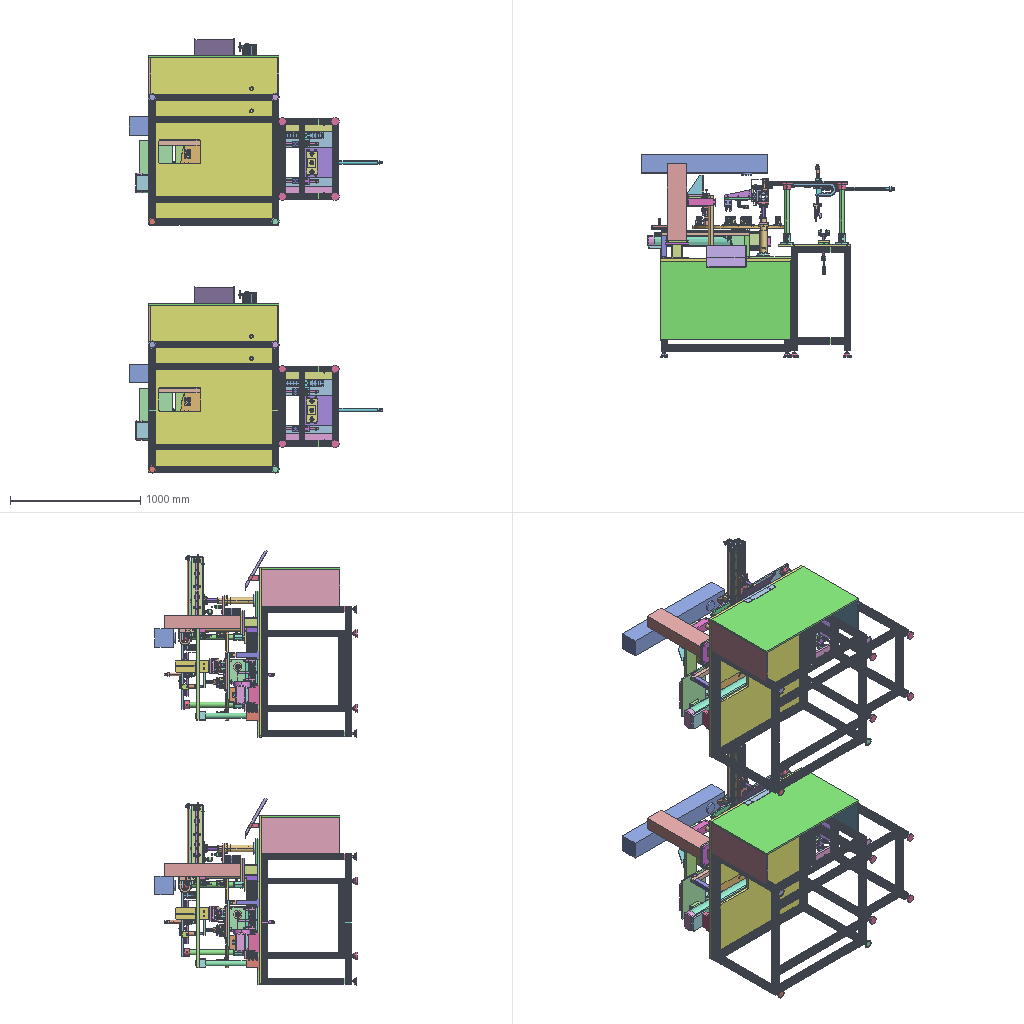Assembly | STEP file | 109 different items | 370 placed | box 1945 x 1552 x 3333 mm
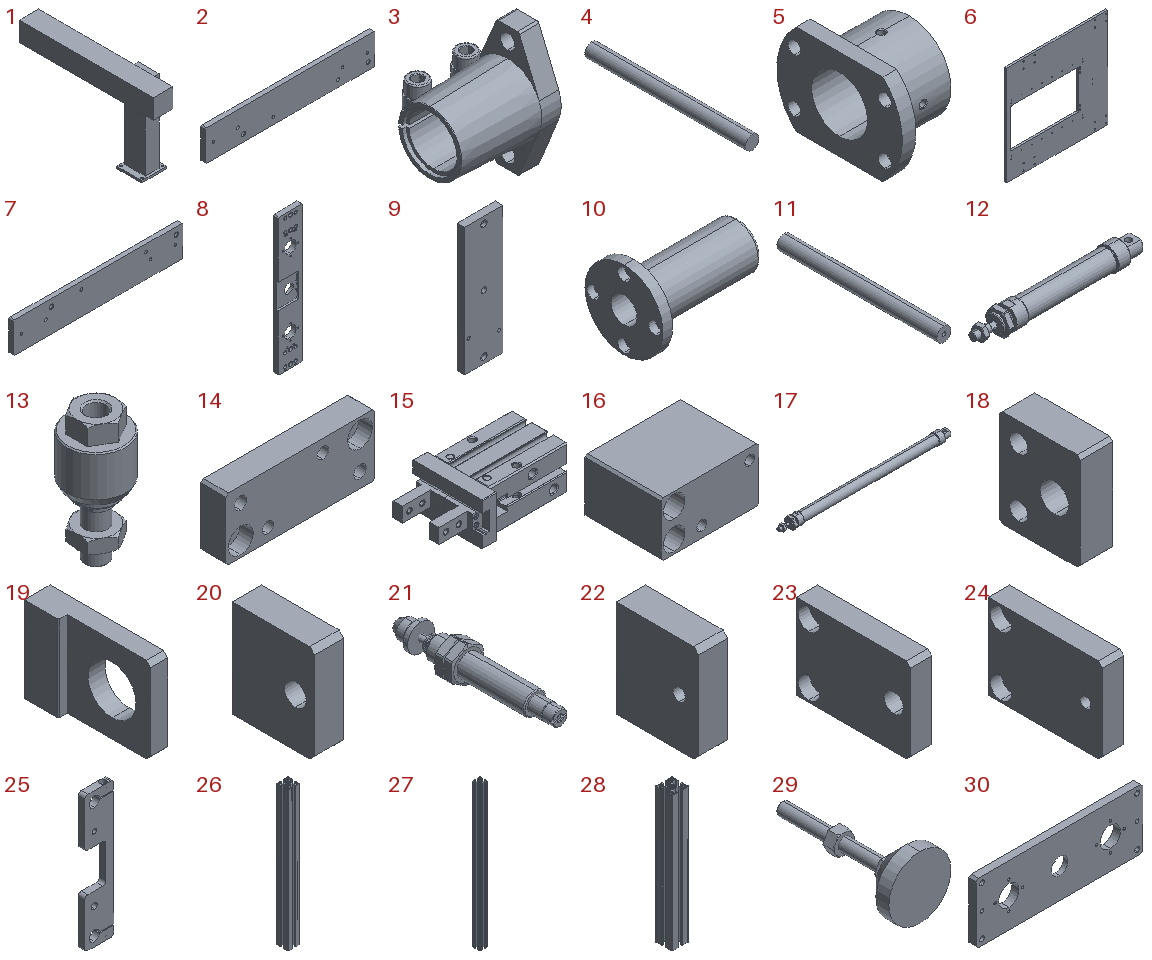Parts list (item | name | quantity | parent item | size | volume):
1 | Ultrasonic welding | x2 | - | 280 x 970 x 675 mm | 28415691 mm3
2 | PN_0058 | x2 | in PN_0042 | 550 x 15 x 100 mm | 808868 mm3
3 | SHFML40 | x8 | in PN_0042 | 80 x 67 x 102 mm | 113573 mm3
4 | PSFJ40-470 | x8 | in PN_0042 | 40 x 470 x 40 mm | 590619 mm3
5 | sthc40 | x8 | in PN_0042 | 50 x 90 x 65 mm | 100252 mm3
6 | PN_0008 | x2 | in PN_0042 | 600 x 12 x 585 mm | 3092667 mm3
7 | PN_0057 | x2 | in PN_0042 | 550 x 15 x 100 mm | 808868 mm3
8 | PN_0025 | x2 | in PN_0042 | 60 x 12 x 335 mm | 203956 mm3
9 | PN_0018 | x2 | in PN_0042 | 60 x 12 x 200 mm | 140928 mm3
10 | LHFRW16 | x4 | in PN_0042 | 70 x 48 x 48 mm | 35245 mm3
11 | PSFJW16-180-M5-N5 | x4 | in PN_0042 | 16 x 180 x 16 mm | 35836 mm3
12 | MA25x75-S (0) | x2 | in PN_0042 | - | -
13 | F-M10125F | x4 | in PN_0042 | 26 x 26 x 58 mm | 16271 mm3
14 | PN_0033 | x2 | in PN_0042 | 60 x 10 x 25 mm | 12893 mm3
15 | HFZ16-CL | x4 | in PN_0042 | 67.3 x 38 x 23.6 mm | 30935 mm3
16 | PN_0049 | x2 | in PN_0042 | 45 x 35 x 25 mm | 32071 mm3
17 | MA25x350-S (0) | x2 | in PN_0042 | - | -
18 | PN_0052 | x2 | in PN_0042 | 10 x 25 x 30 mm | 5805 mm3
19 | PN_0027 | x2 | in PN_0042 | 12 x 55 x 40 mm | 16587 mm3
20 | PN_0024 | x2 | in PN_0042 | 12 x 34 x 40 mm | 15028 mm3
21 | ACJ-1007 | x6 | in PN_0042 | - | -
22 | PN_0037 | x2 | in PN_0042 | 12 x 34 x 40 mm | 15555 mm3
23 | PN_0007 | x2 | in PN_0042 | 10 x 54 x 40 mm | 19857 mm3
24 | PN_0015 | x2 | in PN_0042 | 10 x 54 x 40 mm | 20297 mm3
25 | PN_0034 | x2 | in PN_0042 | 45 x 10 x 210 mm | 67263 mm3
26 | PN_0041 | x10 | in PN_0003 | 45 x 45 x 530 mm | 340057 mm3
27 | PN_0017 | x8 | in PN_0003 | 45 x 45 x 800 mm | 513293 mm3
28 | PN_0029 | x8 | in PN_0003 | 45 x 45 x 360 mm | 230982 mm3
29 | FBR60-12-100 | x8 | in PN_0003 | 60 x 133 x 60 mm | 73980 mm3
30 | PN_0016 | x2 | in PN_0028 | 230 x 10 x 83 mm | 156846 mm3
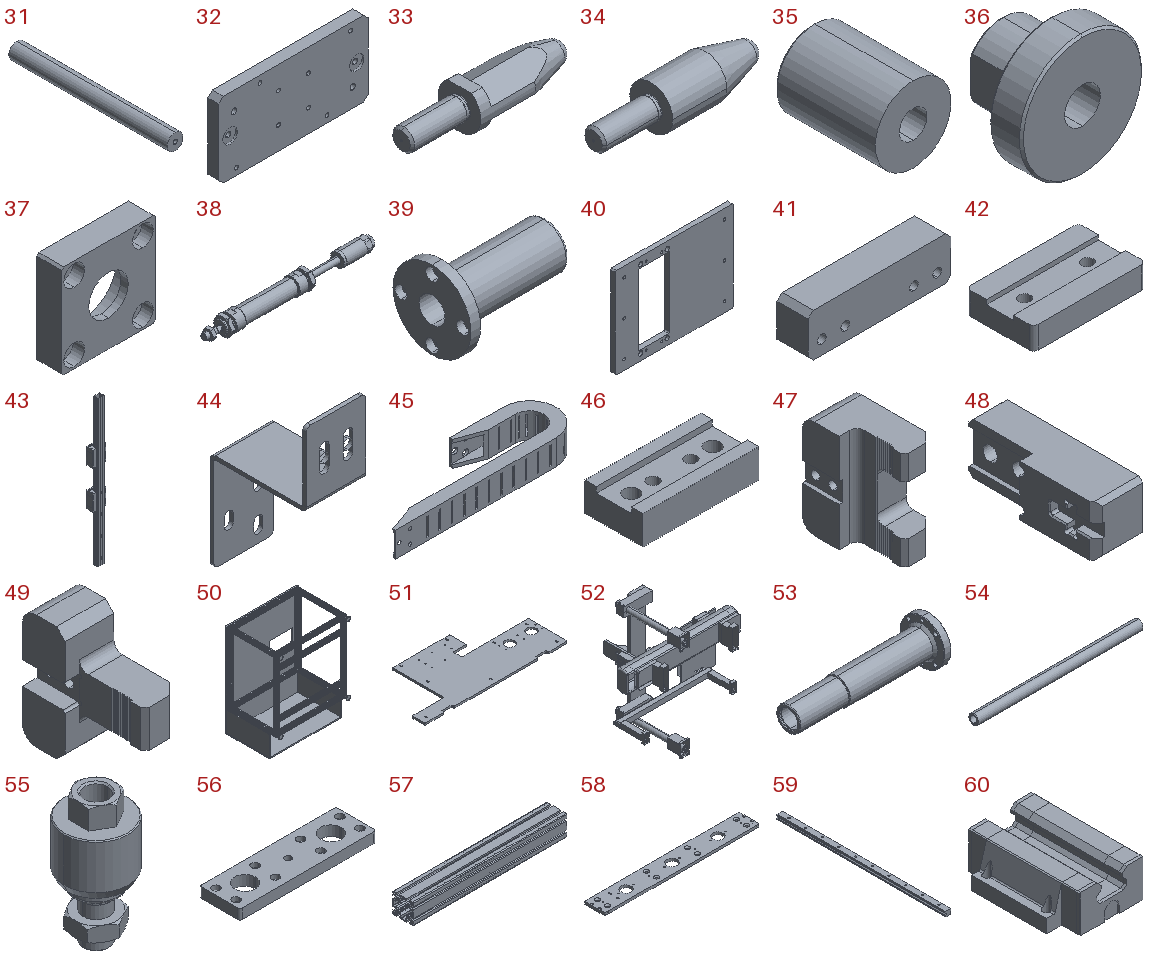31 | PSFJW16-160-M5-N5 | x4 | in PN_0028 | 16 x 160 x 16 mm | 31815 mm3
32 | PN_0056 | x2 | in PN_0028 | 165 x 12 x 83 mm | 159860 mm3
33 | FLNND6_P11_8_B15_0_L10_FLNND6-P11.8-B15.0-L10 | x2 | in PN_0028 | 44.415 x 11.8 x 10.8 mm | 2279 mm3
34 | FLNNA6_P11_9_B15_0_L10---2_FLNNA6-P11.9-B15.0-L10 | x2 | in PN_0028 | 44.601 x 11.9 x 11.9 mm | 2879 mm3
35 | PN_0011 | x8 | in PN_0028 | 15 x 20 x 15 mm | 2655 mm3
36 | PN_0022 | x2 | in PN_0028 | 30 x 20 x 30 mm | 7262 mm3
37 | PN_0055 | x2 | in PN_0028 | 45 x 12 x 45 mm | 14544 mm3
38 | MAJ-25x50-30-S (0300) | x2 | in PN_0028 | - | -
39 | LHFRW16-2 | x4 | in PN_0028 | 70 x 48 x 48 mm | 35245 mm3
40 | PN_0021 | x2 | in PN_0042 | 300 x 12 x 230 mm | 646136 mm3
41 | PN_0043 | x4 | in PN_0042 | 83 x 18 x 25 mm | 35337 mm3
42 | PN_0044 | x2 | in PN_0042 | 50 x 30 x 10 mm | 13429 mm3
43 | EHG20SA | x4 | in PN_0042 | - | -
44 | PN_0005 | x2 | in PN_0042 | - | -
45 | TP18.35(Ruiao) | x2 | in PN_0042 | 349.5 x 99 x 47 mm | 205052 mm3
46 | PN_0031 | x4 | in PN_0042 | 40 x 20 x 10 mm | 6491 mm3
47 | PN_0053 | x2 | in PN_0042 | 19.2 x 35 x 39.94 mm | 17498 mm3
48 | PN_0051 | x4 | in PN_0042 | 11 x 33 x 12 mm | 3442 mm3
49 | PN_0002 | x2 | in PN_0042 | 17 x 38.5 x 40 mm | 12649 mm3
50 | Final inspection modification | x2 | - | 1005 x 750 x 1303 mm | 47486474 mm3
51 | PN_0001 | x2 | - | 1120 x 505 x 15 mm | 5379555 mm3
52 | PN_0054 | x2 | - | - | -
53 | PN_0061_Default<machined> | x4 | in PN_0020 | 292 x 92 x 92 mm | 411633 mm3
54 | PSPJ30_X_PSPJ25-400 | x4 | in PN_0020 | 500 x 30 x 30 mm | 196257 mm3
55 | F_M14150F_F-M14150F-P | x2 | in PN_0020 | 34.5 x 34.5 x 70 mm | 35537 mm3
56 | PN_0006 | x2 | in PN_0020 | 270 x 80 x 20 mm | 358346 mm3
57 | PN_0062_Default<machined> | x2 | in PN_0020 | 606 x 80 x 80 mm | 921943 mm3
58 | PN_0050 | x2 | in PN_0020 | 606 x 80 x 10 mm | 436139 mm3
59 | HGW20CC guide rail-x1 | x2 | in PN_0020 | 20 x 606 x 17.5 mm | 184749 mm3
60 | HGW20CC | x2 | in PN_0020 | 63 x 75 x 25.4 mm | 76452 mm3
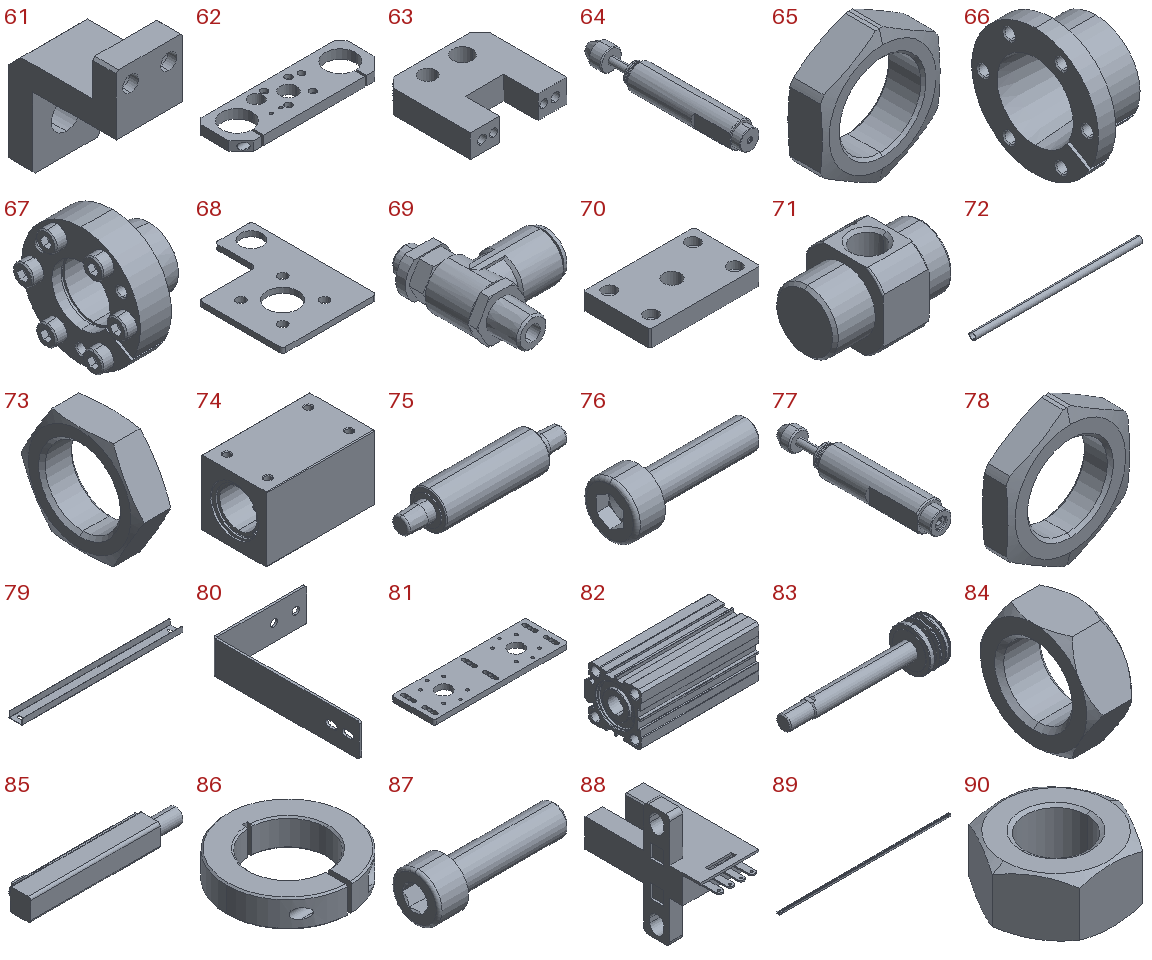61 | PN_0030 | x2 | in PN_0020 | 28 x 45 x 55 mm | 22140 mm3
62 | PN_0048 | x2 | in PN_0020 | 240 x 76 x 15 mm | 181438 mm3
63 | PN_0010 | x4 | in PN_0020 | 50 x 45 x 12 mm | 17113 mm3
64 | ACA_1412_1_Body | x6 | in ACA_1412_1_ACA-1412-1 | 14 x 90 x 14 mm | 10670 mm3
65 | ACA_1412_1_NT | x12 | in ACA_1412_1_ACA-1412-1 | 19 x 6 x 21.289 mm | 1012 mm3
66 | MLR30body | x4 | in MLR30_MLR30 | 28 x 58.56 x 58.56 mm | 23041 mm3
67 | MLR30bonnet | x4 | in MLR30_MLR30 | 41 x 61 x 61 mm | 20958 mm3
68 | PN_0060 | x4 | in PN_0020 | 90 x 120 x 5 mm | 36578 mm3
69 | SPCNL8_1_B_SPCNL8-1-B | x4 | in PN_0020 | 32.883 x 41.9 x 15 mm | 6567 mm3
70 | PN_0035 | x2 | in PN_0020 | 66 x 40 x 10 mm | 24322 mm3
71 | RMS20X50_FCV | x4 | - | 38 x 25 x 25 mm | 12617 mm3
72 | - | x2 | - | 576 x 23 x 23 mm | 58326 mm3
73 | RMS20X50_Nut | x4 | - | 8 x 30.022 x 26 mm | 2480 mm3
74 | RMS20X50_Body | x4 | in PN_0020 | 66 x 40 x 40 mm | 76860 mm3
75 | RMS20X50_Piston | x2 | - | 86 x 20 x 20 mm | 19878 mm3
76 | hexagon socket head cap screws gb_PreviewCfg | x8 | in PN_0020 | 7.6 x 3 x 3 mm | 21.652 mm3
77 | ACA_1210_1_Body | x4 | in ACA_1210_1_ACA-1210-1 | 12 x 67 x 12 mm | 5400 mm3
78 | ACA_1210_1_NT | x8 | in ACA_1210_1_ACA-1210-1 | 17 x 4 x 19.048 mm | 576.274 mm3
79 | PN_0040 | x2 | in PN_0020 | 580 x 47.4 x 21.2 mm | 59564 mm3
80 | PN_0032 | x2 | in PN_0020 | 84 x 134 x 30 mm | 12571 mm3
81 | PN_0036 | x2 | in PN_0020 | - | -
82 | ACQS_40x8080_b | x2 | - | 119.5 x 57 x 53 mm | 166175 mm3
83 | ACQS_40x80_B_80r | x2 | - | 143 x 40 x 40 mm | 43643 mm3
84 | ACQ_40_Nut | x2 | - | 8 x 21.939 x 19 mm | 1486 mm3
85 | CS1_G | x4 | - | 30.5 x 5.5 x 4.4 mm | 552.742 mm3
86 | SCSJ50_18b | x2 | in SCSJ50_18_SCSJ50-18 | 80 x 79.972 x 18 mm | 50835 mm3
87 | - | x2 | in SCSJ50_18_SCSJ50-18 | 38 x 13 x 13 mm | 2398 mm3
88 | EE-SX672-D12d(Omron U-shaped photoelectric) | x4 | in PN_0020 | 13.5 x 28.5 x 26 mm | 1979 mm3
89 | SENAK3-X | x2 | in PN_0020 | 606 x 9 x 6 mm | 19051 mm3
90 | hex nuts 1-fine pitch-grades ab gb_PreviewCfg | x2 | in PN_0020 | 18.475 x 16 x 8.4 mm | 1301 mm3
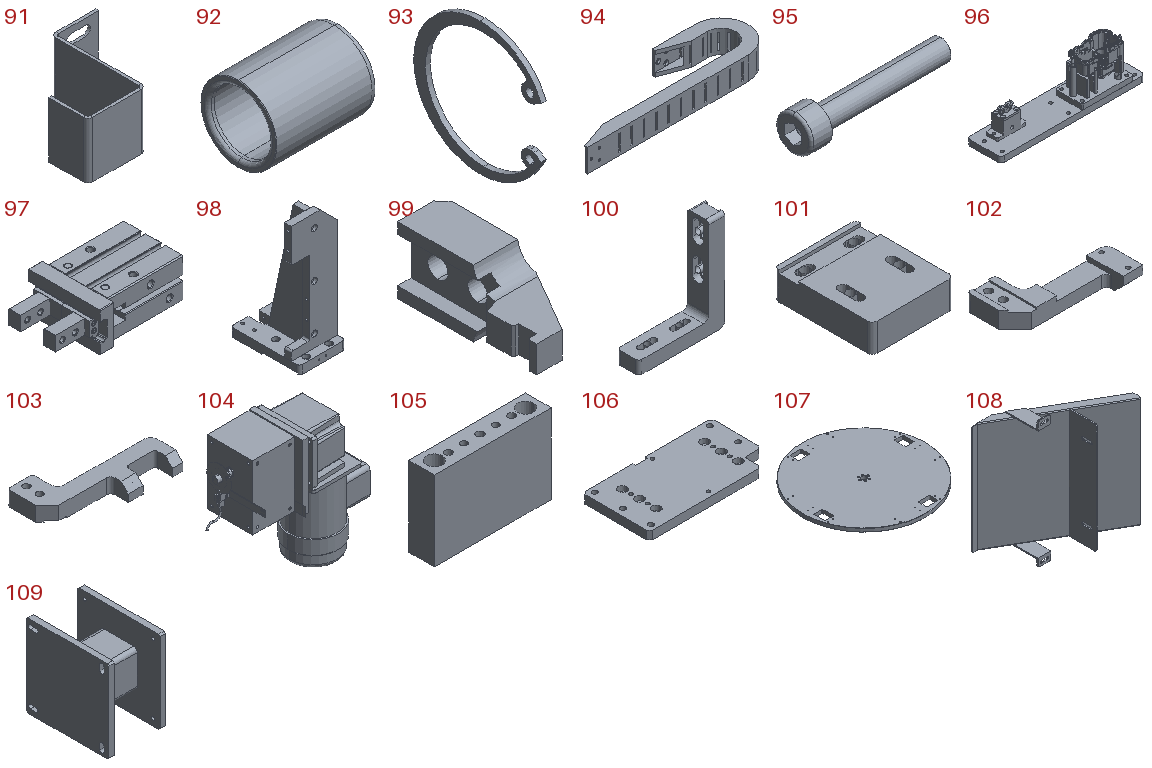91 | PN_0038 | x2 | in PN_0020 | 35.75 x 33 x 20 mm | 1529 mm3
92 | MPBZ30_50_MPBZ30-50 | x8 | in PN_0020 | 50 x 38 x 38 mm | 21031 mm3
93 | RTWN37_RTWN37 | x8 | in PN_0020 | 1.5 x 38.283 x 39.8 mm | 431.748 mm3
94 | TP15.30(Ruiao) | x2 | in PN_0020 | 349.5 x 99 x 43 mm | 233329 mm3
95 | GB_Hex socket head cylinder screw_M5X30_M5X30 | x2 | in PN_0020 | 35 x 8.5 x 8.5 mm | 830.962 mm3
96 | PN_0047 | x10 | in PN_0020, Turntable carrier | - | -
97 | HFZ20_CL_ | x4 | in PN_0020 | 84.7 x 50 x 27.6 mm | 63972 mm3
98 | PN_0013 | x2 | in PN_0020 | 80 x 120 x 219 mm | 332786 mm3
99 | PN_0004 | x4 | in PN_0020 | 13.8 x 35 x 15 mm | 2765 mm3
100 | PN_0023 | x2 | in PN_0020 | - | -
101 | PN_0019 | x2 | in PN_0020 | - | -
102 | PN_0059 | x2 | in PN_0020 | 67.5 x 39 x 10 mm | 9820 mm3
103 | PN_0045 | x2 | in PN_0020 | 80 x 39 x 10 mm | 11727 mm3
104 | PN_0046 | x2 | in PN_0014 | - | -
105 | PN_0026 | x4 | in PN_0014 | 110 x 24 x 75 mm | 174240 mm3
106 | PN_0012 | x2 | in PN_0014 | 230 x 120 x 15 mm | 374023 mm3
107 | PN_0009 | x2 | in Turntable carrier | 700 x 700 x 20 mm | 7409055 mm3
108 | PN_0039 | x2 | - | 305 x 168 x 349 mm | 258678 mm3
109 | PN_0063_Default<machined> | x2 | - | 124 x 180 x 180 mm | 884667 mm3
Placements (level | parent | child | x y z in mm | rotation matrix by rows), first 340 of 402 lines:
1 | subassembly 2 | Ultrasonic welding | -163.522 990.0 690.769 | 0 1 0 0 0 1 1 0 0
1 | subassembly 2 | PN_0042 | 719.818 434.3 178.269 | 1 0 0 0 1 0 0 0 1
2 | PN_0042 | PN_0058 | -40.835 -5.8 -0.0 | 1 0 0 0 1 0 0 0 1
2 | PN_0042 | SHFML40 | 169.165 9.2 -0.0 | 0 0 -1 -1 0 0 0 1 0
2 | PN_0042 | PSFJ40-470 | 169.165 9.2 0.0 | 0.9999 0 -0.01343 0 1 0 0.01343 0 0.9999
2 | PN_0042 | sthc40 | 169.165 479.2 -0.0 | 0 1 0 -1 0 0 0 0 1
2 | PN_0042 | PN_0008 | -85.835 479.2 260.0 | 1 0 0 0 1 0 0 0 1
2 | PN_0042 | PN_0057 | -40.835 -5.8 520.0 | 1 0 0 0 1 0 0 0 1
2 | PN_0042 | PN_0025 | -14.335 451.2 232.5 | 1 0 0 0 1 0 0 0 1
2 | PN_0042 | PN_0018 | -14.335 322.2 232.5 | 1 0 0 0 1 0 0 0 1
2 | PN_0042 | LHFRW16 | -14.335 457.2 322.5 | 0 1 0 -1 0 0 0 0 1
2 | PN_0042 | PSFJW16-180-M5-N5 | -14.335 320.2 322.5 | 0.998 0 -0.06356 0 1 0 0.06356 0 0.998
2 | PN_0042 | MA25x75-S (0) | -14.335 467.2 232.5 | 0 0 1 1 0 0 0 1 0
2 | PN_0042 | F-M10125F | -14.335 357.2 232.5 | 0.7177 0.6964 0 0 0 1 0.6964 -0.7177 0
2 | PN_0042 | PN_0033 | -14.335 300.2 173.0 | 1 0 0 0 1 0 0 0 1
2 | PN_0042 | HFZ16-CL | -16.335 300.2 173.0 | 0 1 0 1 0 0 0 0 -1
2 | PN_0042 | HFZ16-CL | -28.835 275.2 308.7 | 0 0 1 1 0 0 0 1 -0
2 | PN_0042 | PN_0049 | -28.835 275.2 301.5 | 0 0 -1 0 1 0 1 0 0
2 | PN_0042 | MA25x350-S (0) | 145.165 434.2 232.5 | 1 0 0 0 -0.8525 0.5227 0 -0.5227 -0.8525
2 | PN_0042 | F-M10125F | 17.665 434.2 232.5 | 0 0 1 -0.03816 -0.9993 0 0.9993 -0.03816 -0
2 | PN_0042 | PN_0052 | 15.665 438.7 232.5 | 1 0 0 0 1 0 0 0 1
2 | PN_0042 | PN_0027 | 123.165 471.2 232.5 | 1 0 0 0 1 0 0 0 1
2 | PN_0042 | PN_0024 | 48.165 471.2 137.5 | 1 0 0 0 1 0 0 0 1
2 | PN_0042 | ACJ-1007 | 81.165 445.2 137.5 | 0 -1 0 0.5268 0 -0.85 0.85 0 0.5268
2 | PN_0042 | PN_0037 | 48.165 471.2 327.5 | 1 0 0 0 1 0 0 0 1
2 | PN_0042 | PN_0007 | -395.835 464.2 137.5 | 1 0 0 0 1 0 0 0 1
2 | PN_0042 | PN_0015 | -395.835 464.2 327.5 | 1 0 0 0 1 0 0 0 1
2 | PN_0042 | ACJ-1007 | -429.835 445.2 137.5 | 0 1 0 0.7993 0 -0.601 -0.601 0 -0.7993
2 | PN_0042 | PN_0034 | -4.335 500.2 232.5 | 1 0 0 0 1 0 0 0 1
2 | PN_0042 | ACJ-1007 | -14.335 515.7 182.5 | 0.986 0 0.1665 0 -1 0 0.1665 0 -0.986
2 | PN_0042 | PN_0003 | 202.398 -37.946 260.0 | 1 0 0 0 1 0 0 0 1
3 | PN_0003 | PN_0041 | -1444.398 -532.32 -265.0 | 1 0 0 0 1 0 0 0 1
3 | PN_0003 | PN_0017 | 551.233 32.146 -1166.165 | 0 -1 0 0 0 -1 1 0 0
3 | PN_0003 | PN_0029 | -13.233 -532.32 -1166.165 | 0 0 -1 0 1 0 1 0 0
3 | PN_0003 | PN_0017 | 551.233 32.146 -1741.165 | 0 -1 0 0 0 -1 1 0 0
3 | PN_0003 | PN_0017 | 146.233 32.146 -1166.165 | 0 -1 0 0 0 -1 1 0 0
3 | PN_0003 | PN_0041 | -1849.398 -577.32 -265.0 | 1 0 0 0 1 0 0 0 1
3 | PN_0003 | PN_0029 | -13.233 -532.32 -1741.165 | 0 0 -1 0 1 0 1 0 0
3 | PN_0003 | PN_0017 | 146.233 32.146 -1741.165 | 0 -1 0 0 0 -1 1 0 0
3 | PN_0003 | PN_0041 | -1444.398 -1237.32 -265.0 | 1 0 0 0 1 0 0 0 1
3 | PN_0003 | PN_0041 | -1849.398 -1237.32 -265.0 | 1 0 0 0 1 0 0 0 1
3 | PN_0003 | PN_0029 | -13.233 -1237.32 -1166.165 | 0 0 -1 0 1 0 1 0 0
3 | PN_0003 | PN_0029 | -13.233 -1237.32 -1741.165 | 0 0 -1 0 1 0 1 0 0
3 | PN_0003 | FBR60-12-100 | 9.267 -817.854 287.5 | 1 0 0 0 1 0 0 0 1
3 | PN_0003 | FBR60-12-100 | 9.267 -817.854 -287.5 | 1 0 0 0 1 0 0 0 1
3 | PN_0003 | FBR60-12-100 | -395.733 -817.854 -287.5 | 1 0 0 0 1 0 0 0 1
3 | PN_0003 | FBR60-12-100 | -395.733 -817.854 287.5 | 1 0 0 0 1 0 0 0 1
3 | PN_0003 | PN_0041 | -1699.398 -532.32 -265.0 | 1 0 0 0 1 0 0 0 1
2 | PN_0042 | PN_0028 | 37.301 24.755 239.519 | 0 0 -1 0 1 0 1 0 0
3 | PN_0028 | PN_0016 | -9.019 -0.5551 5.136 | 1 0 0 0 1 0 0 0 1
3 | PN_0028 | PSFJW16-160-M5-N5 | 60.981 -102.555 5.136 | 1 0 0 0 1 0 0 0 1
3 | PN_0028 | PSFJW16-160-M5-N5 | -79.019 -102.555 5.136 | 1 0 0 0 1 0 0 0 1
3 | PN_0028 | PN_0056 | -9.019 55.445 5.136 | 1 0 0 0 1 0 0 0 1
3 | PN_0028 | FLNND6_P11_8_B15_0_L10_FLNND6-P11.8-B15.0-L10 | 56.481 67.445 -15.864 | 0 -1 0 1 0 0 0 0 1
3 | PN_0028 | FLNNA6_P11_9_B15_0_L10---2_FLNNA6-P11.9-B15.0-L10 | -74.519 67.445 26.137 | 0 -1 0 1 0 0 0 0 1
3 | PN_0028 | PN_0011 | 27.981 67.445 -28.863 | 1 0 0 0 1 0 0 0 1
3 | PN_0028 | PN_0011 | -46.019 67.445 39.136 | 1 0 0 0 1 0 0 0 1
3 | PN_0028 | PN_0011 | -72.019 67.445 -28.863 | 1 0 0 0 1 0 0 0 1
3 | PN_0028 | PN_0011 | 53.981 67.445 39.136 | 1 0 0 0 1 0 0 0 1
3 | PN_0028 | PN_0022 | -9.019 55.445 5.136 | 0.7332 0 0.68 0 -1 0 0.68 0 -0.7332
3 | PN_0028 | PN_0055 | -9.019 43.445 5.136 | 1 0 0 0 1 0 0 0 1
3 | PN_0028 | MAJ-25x50-30-S (0300) | -9.019 -16.555 5.136 | 0 0 -1 -1 0 0 0 1 0
3 | PN_0028 | LHFRW16-2 | 60.981 15.445 5.136 | 0 1 0 -1 0 0 0 0 1
3 | PN_0028 | LHFRW16-2 | -79.019 15.445 5.136 | 0 1 0 -1 0 0 0 0 1
2 | PN_0042 | PN_0021 | 84.165 -5.8 230.5 | 1 0 0 0 1 0 0 0 1
2 | PN_0042 | PN_0043 | 32.165 6.2 333.0 | 1 0 0 0 1 0 0 0 1
2 | PN_0042 | PN_0043 | 32.165 6.2 128.0 | -1 0 0 0 1 0 0 0 -1
2 | PN_0042 | PN_0044 | 123.165 479.2 232.5 | 0 1 0 0 0 -1 -1 0 -0
2 | PN_0042 | EHG20SA | -434.835 472.098 376.317 | 0 0 -1 0 -1 0 -1 0 -0
2 | PN_0042 | EHG20SA | -434.835 472.098 91.317 | 0 0 -1 0 -1 0 -1 0 -0
2 | PN_0042 | PN_0005 | -4.335 406.7 397.5 | 1 0 0 0 -1 0 0 0 -1
2 | PN_0042 | TP18.35(Ruiao) | -224.335 467.7 440.5 | 1 0 0 0 -1 0 0 0 -1
2 | PN_0042 | PN_0031 | 48.165 479.2 327.5 | 0 -1 0 0 0 -1 1 0 -0
2 | PN_0042 | PN_0031 | 48.165 479.2 137.5 | 0 -1 0 0 0 -1 1 0 -0
2 | PN_0042 | SHFML40 | -250.835 9.2 0.0 | 0 0 -1 -1 0 0 0 1 0
2 | PN_0042 | SHFML40 | 169.165 9.2 520.0 | 0 0 -1 -1 0 0 0 1 0
2 | PN_0042 | SHFML40 | -250.835 9.2 520.0 | 0 0 -1 -1 0 0 0 1 0
2 | PN_0042 | sthc40 | -250.835 479.2 -0.0 | 0 1 0 -1 0 0 0 0 1
2 | PN_0042 | sthc40 | 169.165 479.2 520.0 | 0 1 0 -1 0 0 0 0 1
2 | PN_0042 | sthc40 | -250.835 479.2 520.0 | 0 1 0 -1 0 0 0 0 1
2 | PN_0042 | PSFJ40-470 | -250.835 9.2 0.0 | 0.9999 0 -0.01343 0 1 0 0.01343 0 0.9999
2 | PN_0042 | PSFJ40-470 | 169.165 9.2 520.0 | 0.9999 0 -0.01343 0 1 0 0.01343 0 0.9999
2 | PN_0042 | PSFJ40-470 | -250.835 9.2 520.0 | 0.9999 0 -0.01343 0 1 0 0.01343 0 0.9999
2 | PN_0042 | PN_0053 | -5.375 232.9 173.03 | 1 0 0 0 1 0 0 0 1
2 | PN_0042 | PN_0051 | -28.835 222.9 326.16 | 0 0 -1 0 1 0 1 0 0
2 | PN_0042 | PN_0002 | -21.595 232.9 173.0 | -1 0 0 0 1 0 0 0 -1
2 | PN_0042 | PN_0051 | -28.835 222.9 291.24 | 0 0 1 0 1 0 -1 0 -0
2 | PN_0042 | PSFJW16-180-M5-N5 | -14.335 320.2 142.5 | 0.998 0 -0.06356 0 1 0 0.06356 0 0.998
2 | PN_0042 | LHFRW16 | -14.335 457.2 142.5 | 0 1 0 -1 0 0 0 0 1
1 | subassembly 2 | Final inspection modification | -1.017 -32.5 911.769 | -1 0 0 0 1 0 0 0 -1
1 | subassembly 2 | PN_0001 | -1.017 345.0 489.269 | 0 -1 0 0 0 -1 1 0 0
1 | subassembly 2 | PN_0054 | -3.106 32.87 911.769 | -1 0 0 0 1 0 0 0 -1
1 | subassembly 2 | PN_0020 | 288.983 477.954 977.897 | 0 0 1 -1 0 0 0 -1 0
2 | PN_0020 | PN_0061_Default<machined> | -171.046 1.128 -0.0 | 1 0 0 0 1 0 0 0 1
2 | PN_0020 | PN_0061_Default<machined> | -171.046 171.128 0.0 | 1 0 0 0 -1 0 0 0 -1
2 | PN_0020 | PSPJ30_X_PSPJ25-400 | -290.379 171.128 -0.0 | 1 0 0 0 0.9961 0.08866 0 -0.08866 0.9961
2 | PN_0020 | PSPJ30_X_PSPJ25-400 | -290.379 1.128 -0.0 | 1 0 0 0 0.9538 0.3006 0 -0.3006 0.9538
2 | PN_0020 | F_M14150F_F-M14150F-P | -277.629 86.128 0.0 | 0 0 1 -0.9375 -0.3479 0 0.3479 -0.9375 0
2 | PN_0020 | PN_0006 | -290.379 86.128 0.0 | 0 0 1 -1 0 0 0 -1 -0
2 | PN_0020 | PN_0062_Default<machined> | -330.379 -26.872 -0.0 | 0 0 1 -1 0 0 0 -1 0
2 | PN_0020 | PN_0050 | -330.379 -26.872 -40.0 | 0 -1 0 -1 0 0 0 0 -1
2 | PN_0020 | HGW20CC guide rail-x1 | -330.379 -64.372 -80.0 | 1 0 0 0 1 0 0 0 1
2 | PN_0020 | HGW20CC | -330.379 204.605 -80.0 | 1 0 0 0 1 0 0 0 1
2 | PN_0020 | PN_0030 | -153.546 48.128 -0.0 | 0 -1 0 1 0 0 0 0 1
2 | PN_0020 | PN_0048 | -116.046 86.128 4.0 | 0 0 -1 1 0 0 0 -1 0
2 | PN_0020 | PN_0010 | -330.379 264.128 -72.5 | 1 0 0 0 0 1 0 -1 0
2 | PN_0020 | PN_0010 | -330.379 -329.872 -72.5 | 1 0 0 0 0 1 0 -1 0
2 | PN_0020 | ACA_1412_1_ACA-1412-1 | -129.546 48.128 -15.0 | 0 -1 0 0.6019 0 0.7986 -0.7986 0 0.6019
3 | ACA_1412_1_ACA-1412-1 | ACA_1412_1_Body | -0.0 -0.0 -0.0 | 1 0 0 0 1 0 0 0 1
3 | ACA_1412_1_ACA-1412-1 | ACA_1412_1_NT | -0.0 46.5 -0.0 | 1 0 0 0 1 0 0 0 1
3 | ACA_1412_1_ACA-1412-1 | ACA_1412_1_NT | -0.0 52.5 -0.0 | 1 0 0 0 1 0 0 0 1
2 | PN_0020 | MLR30_MLR30 | -254.379 1.128 0.0 | -1 0 0 0 -0.8293 -0.5589 0 -0.5589 0.8293
3 | MLR30_MLR30 | MLR30body | -0.0 -0.0 -0.0 | 1 0 0 0 1 0 0 0 1
3 | MLR30_MLR30 | MLR30bonnet | -0.0 -0.0 -0.0 | 1 0 0 0 1 0 0 0 1
2 | PN_0020 | MLR30_MLR30 | -254.379 171.128 -0.0 | -1 0 0 0 -0.5264 0.8502 0 0.8502 0.5264
3 | MLR30_MLR30 | MLR30body | -0.0 -0.0 -0.0 | 1 0 0 0 1 0 0 0 1
3 | MLR30_MLR30 | MLR30bonnet | -0.0 -0.0 -0.0 | 1 0 0 0 1 0 0 0 1
2 | PN_0020 | PN_0060 | -350.379 276.128 0.0 | 0 -1 0 0 0 1 -1 0 0
2 | PN_0020 | PN_0060 | -350.379 -334.872 0.0 | 0 -1 0 0 0 1 -1 0 0
2 | PN_0020 | SPCNL8_1_B_SPCNL8-1-B | -395.379 268.628 -63.0 | -1 0 0 0 0 -1 0 -1 -0
2 | PN_0020 | SPCNL8_1_B_SPCNL8-1-B | -395.379 -322.372 -63.0 | -1 0 0 0 0 -1 0 -1 -0
2 | PN_0020 | PN_0035 | -395.379 204.605 -55.0 | 0 -1 0 -1 0 0 0 0 -1
2 | PN_0020 | subassembly 3 | -395.379 261.128 -35.0 | 0 -1 0 -1 0 0 0 0 -1
3 | subassembly 3 | RMS20X50_FCV | -0.0 -0.0 -0.0 | 1 0 0 0 1 0 0 0 1
3 | subassembly 3 | subassembly 4 | -0.0 -0.0 -0.0 | 1 0 0 0 1 0 0 0 1
3 | subassembly 3 | RMS20X50_FCV | 576.0 0.0 -0.0 | -1 0 0 0 -1 0 0 0 1
3 | subassembly 3 | RMS20X50_Nut | 599.0 0.0 -0.0 | -1 0 0 0 -1 0 0 0 1
3 | subassembly 3 | RMS20X50_Body | 5.0 0.0 -0.0 | 1 0 0 0 1 0 0 0 1
3 | subassembly 3 | RMS20X50_Piston | 10.0 0.0 -0.0 | 1 0 0 0 1 0 0 0 1
3 | subassembly 3 | RMS20X50_Nut | -23.0 0.0 -0.0 | 1 0 0 0 1 0 0 0 1
2 | PN_0020 | RMS20X50_Body | -395.379 237.605 -35.0 | 0 -1 0 -1 0 0 0 0 -1
2 | PN_0020 | hexagon socket head cap screws gb_PreviewCfg | -395.379 204.605 -92.0 | 0 -0.3327 0.943 0 -0.943 -0.3327 1 0 -0
2 | PN_0020 | ACA_1210_1_ACA-1210-1 | -322.379 299.628 -87.0 | 0.9765 0 0.2154 0 -1 0 0.2154 0 -0.9765
3 | ACA_1210_1_ACA-1210-1 | ACA_1210_1_Body | -0.0 -0.0 -0.0 | 1 0 0 0 1 0 0 0 1
3 | ACA_1210_1_ACA-1210-1 | ACA_1210_1_NT | 0.0 32.5 -0.0 | 1 0 0 0 1 0 0 0 1
3 | ACA_1210_1_ACA-1210-1 | ACA_1210_1_NT | 0.0 36.5 -0.0 | 1 0 0 0 1 0 0 0 1
2 | PN_0020 | ACA_1210_1_ACA-1210-1 | -322.379 -353.372 -87.0 | 0.4428 0 0.8966 0 1 0 -0.8966 0 0.4428
3 | ACA_1210_1_ACA-1210-1 | ACA_1210_1_Body | -0.0 -0.0 -0.0 | 1 0 0 0 1 0 0 0 1
3 | ACA_1210_1_ACA-1210-1 | ACA_1210_1_NT | 0.0 32.5 -0.0 | 1 0 0 0 1 0 0 0 1
3 | ACA_1210_1_ACA-1210-1 | ACA_1210_1_NT | 0.0 36.5 -0.0 | 1 0 0 0 1 0 0 0 1
2 | PN_0020 | hexagon socket head cap screws gb_PreviewCfg | -340.379 232.628 -87.0 | 0 -0.3713 0.9285 1 0 0 0 0.9285 0.3713
2 | PN_0020 | hexagon socket head cap screws gb_PreviewCfg | -340.379 -286.372 -87.0 | 0 -0.6192 0.7853 -1 0 0 0 -0.7853 -0.6192
2 | PN_0020 | PN_0040 | -371.579 -13.872 16.3 | 0 0 -1 -1 0 0 0 1 -0
2 | PN_0020 | PN_0032 | -420.786 229.605 -94.0 | 1 0 0 0 0 1 0 -1 0
2 | PN_0020 | PN_0036 | 120.954 86.128 0.0 | 0 0 1 1 0 0 0 1 0
2 | PN_0020 | hexagon socket head cap screws gb_PreviewCfg | -118.646 122.128 -15.0 | 1 0 0 0 1 0 0 0 1
2 | PN_0020 | ACA_1412_1_ACA-1412-1 | -129.546 48.128 -15.0 | 0 -1 0 1 0 0 0 0 1
3 | ACA_1412_1_ACA-1412-1 | ACA_1412_1_Body | -0.0 -0.0 -0.0 | 1 0 0 0 1 0 0 0 1
3 | ACA_1412_1_ACA-1412-1 | ACA_1412_1_NT | -0.0 46.5 -0.0 | 1 0 0 0 1 0 0 0 1
3 | ACA_1412_1_ACA-1412-1 | ACA_1412_1_NT | -0.0 52.5 -0.0 | 1 0 0 0 1 0 0 0 1
2 | PN_0020 | subassembly 5 | -116.046 86.128 0.0 | 1 0 0 0 1 0 0 0 1
3 | subassembly 5 | ACQS_40x8080_b | -0.0 -0.0 -0.0 | 1 0 0 0 0 -1 0 1 0
3 | subassembly 5 | ACQS_40x80_B_80r | -0.0 -0.0 -0.0 | 1 0 0 0 1 0 0 0 1
3 | subassembly 5 | ACQ_40_Nut | -14.25 -0.0 -0.0 | -1 0 0 0 -1 0 0 0 1
3 | subassembly 5 | CS1_G | 1.0 9.931 21.298 | 1 0 0 0 0.4226 -0.9063 0 0.9063 0.4226
3 | subassembly 5 | CS1_G | 118.5 -9.931 21.298 | -1 0 0 0 -0.4226 0.9063 0 0.9063 0.4226
2 | PN_0020 | SCSJ50_18_SCSJ50-18 | -107.046 1.128 -0.0 | 0 0 1 0 -1 0 1 0 0
3 | SCSJ50_18_SCSJ50-18 | SCSJ50_18b | -0.0 -0.0 -0.0 | 1 0 0 0 1 0 0 0 1
3 | SCSJ50_18_SCSJ50-18 | subassembly 6 | 15.0 -32.0 -0.0 | -1 0 0 0 -1 0 0 0 1
2 | PN_0020 | EE-SX672-D12d(Omron U-shaped photoelectric) | -280.129 118.128 -56.75 | 0 1 0 0 0 -1 -1 0 0
2 | PN_0020 | SENAK3-X | -285.879 176.128 -44.0 | 0 -1 0 -1 0 0 0 0 -1
2 | PN_0020 | EE-SX672-D12d(Omron U-shaped photoelectric) | -280.129 -281.622 -56.75 | 0 1 0 0 0 -1 -1 0 0
2 | PN_0020 | ACA_1412_1_ACA-1412-1 | -129.546 48.128 -15.0 | 0 -1 0 0.8791 0 -0.4767 0.4767 0 0.8791
3 | ACA_1412_1_ACA-1412-1 | ACA_1412_1_Body | -0.0 -0.0 -0.0 | 1 0 0 0 1 0 0 0 1
3 | ACA_1412_1_ACA-1412-1 | ACA_1412_1_NT | -0.0 46.5 -0.0 | 1 0 0 0 1 0 0 0 1
3 | ACA_1412_1_ACA-1412-1 | ACA_1412_1_NT | -0.0 52.5 -0.0 | 1 0 0 0 1 0 0 0 1
2 | PN_0020 | hex nuts 1-fine pitch-grades ab gb_PreviewCfg | -340.379 -317.872 -87.0 | 0.5037 -0.8639 0 0 0 -1 0.8639 0.5037 -0
2 | PN_0020 | PN_0038 | -262.786 204.605 -56.25 | 0 -1 0 0 0 1 -1 0 -0
2 | PN_0020 | MPBZ30_50_MPBZ30-50 | -166.046 1.128 -0.0 | 1 0 0 0 0.7589 0.6512 0 -0.6512 0.7589
2 | PN_0020 | MPBZ30_50_MPBZ30-50 | -166.046 171.128 0.0 | 1 0 0 0 0.2659 0.964 0 -0.964 0.2659
2 | PN_0020 | MPBZ30_50_MPBZ30-50 | 63.954 1.128 0.0 | 1 0 0 0 0.6815 -0.7318 0 0.7318 0.6815
2 | PN_0020 | MPBZ30_50_MPBZ30-50 | 63.954 171.128 0.0 | 1 0 0 0 0.6815 -0.7318 0 0.7318 0.6815
2 | PN_0020 | RTWN37_RTWN37 | -166.896 1.128 -0.0 | 1 0 0 0 0.6761 -0.7368 0 0.7368 0.6761
2 | PN_0020 | RTWN37_RTWN37 | -166.896 171.128 0.0 | 1 0 0 0 0.5147 -0.8574 0 0.8574 0.5147
2 | PN_0020 | RTWN37_RTWN37 | 114.804 1.128 -0.0 | 1 0 0 0 -0.9964 -0.08438 0 0.08438 -0.9964
2 | PN_0020 | RTWN37_RTWN37 | 114.804 171.128 0.0 | 1 0 0 0 -0.9964 -0.08438 0 0.08438 -0.9964
2 | PN_0020 | TP15.30(Ruiao) | -383.079 -5.395 17.3 | 0 -1 0 1 0 0 0 0 1
2 | PN_0020 | GB_Hex socket head cylinder screw_M5X30_M5X30 | -337.554 193.128 -84.5 | 0 -0.2637 -0.9646 1 0 0 0 -0.9646 0.2637
2 | PN_0020 | PN_0047 | -0.2834 815.301 3543.794 | 0 0 -1 0 1 0 1 0 -0
2 | PN_0020 | HFZ20_CL_ | -316.836 273.405 -271.0 | -1 0 0 0 0 -1 0 -1 0
2 | PN_0020 | PN_0013 | -355.786 204.605 -77.0 | 0 -1 0 -1 0 0 0 0 -1
2 | PN_0020 | PN_0004 | -252.136 265.905 -268.41 | 0 -1 0 0 0 1 -1 0 -0
2 | PN_0020 | PN_0004 | -252.136 280.905 -273.59 | 0 -1 0 0 0 -1 1 0 0
2 | PN_0020 | HFZ20_CL_ | -344.786 257.605 -189.2 | -1 0 0 0 1 0 0 0 -1
2 | PN_0020 | PN_0023 | -315.786 250.605 -215.0 | 0 1 0 -1 0 0 0 0 1
2 | PN_0020 | PN_0019 | -294.836 259.605 -271.0 | 0 -1 0 0 0 -1 1 0 0
2 | PN_0020 | PN_0059 | -264.586 282.765 -163.5 | 0 -1 0 0 0 -1 1 0 0
2 | PN_0020 | PN_0045 | -259.586 242.445 -157.25 | 0 -1 0 0 0 -1 1 0 0
1 | subassembly 2 | PN_0014 | 195.047 506.863 362.055 | 1 0 0 0 1 0 0 0 1
2 | PN_0014 | PN_0046 | -99.074 48.137 46.714 | 1 0 0 0 1 0 0 0 1
2 | PN_0014 | PN_0026 | -99.074 -109.363 149.714 | 1 0 0 0 0 -1 0 1 0
2 | PN_0014 | PN_0026 | -99.074 -109.363 3.714 | 1 0 0 0 0 -1 0 1 0
2 | PN_0014 | PN_0012 | -99.074 -154.363 76.714 | 0 -1 0 0 0 -1 1 0 -0
2 | PN_0014 | Turntable carrier | -184.189 -38.664 -46.095 | 0 -1 0 0 0 1 -1 0 0
3 | Turntable carrier | PN_0009 | -92.809 -85.115 96.8 | 1 0 0 0 1 0 0 0 1
3 | Turntable carrier | PN_0047 | 3643.995 161.058 10.038 | 1 0 0 0 1 0 0 0 1
3 | Turntable carrier | PN_0047 | 153.364 -3821.92 10.038 | 0 1 0 -1 0 0 0 0 1
3 | Turntable carrier | PN_0047 | -3829.614 -331.289 10.038 | -1 0 0 0 -1 0 0 0 1
3 | Turntable carrier | PN_0047 | -338.982 3651.689 10.038 | 0 -1 0 1 0 0 0 0 1
1 | subassembly 2 | PN_0042 | 719.818 434.3 2078.269 | 1 0 0 0 1 0 0 0 1
2 | PN_0042 | PN_0058 | -40.835 -5.8 -0.0 | 1 0 0 0 1 0 0 0 1
2 | PN_0042 | SHFML40 | 169.165 9.2 -0.0 | 0 0 -1 -1 0 0 0 1 0
2 | PN_0042 | PSFJ40-470 | 169.165 9.2 0.0 | 0.9999 0 -0.01343 0 1 0 0.01343 0 0.9999
2 | PN_0042 | sthc40 | 169.165 479.2 -0.0 | 0 1 0 -1 0 0 0 0 1
2 | PN_0042 | PN_0008 | -85.835 479.2 260.0 | 1 0 0 0 1 0 0 0 1
2 | PN_0042 | PN_0057 | -40.835 -5.8 520.0 | 1 0 0 0 1 0 0 0 1
2 | PN_0042 | PN_0025 | -14.335 451.2 232.5 | 1 0 0 0 1 0 0 0 1
2 | PN_0042 | PN_0018 | -14.335 322.2 232.5 | 1 0 0 0 1 0 0 0 1
2 | PN_0042 | LHFRW16 | -14.335 457.2 322.5 | 0 1 0 -1 0 0 0 0 1
2 | PN_0042 | PSFJW16-180-M5-N5 | -14.335 320.2 322.5 | 0.998 0 -0.06356 0 1 0 0.06356 0 0.998
2 | PN_0042 | MA25x75-S (0) | -14.335 467.2 232.5 | 0 0 1 1 0 0 0 1 0
2 | PN_0042 | F-M10125F | -14.335 357.2 232.5 | 0.7177 0.6964 0 0 0 1 0.6964 -0.7177 0
2 | PN_0042 | PN_0033 | -14.335 300.2 173.0 | 1 0 0 0 1 0 0 0 1
2 | PN_0042 | HFZ16-CL | -16.335 300.2 173.0 | 0 1 0 1 0 0 0 0 -1
2 | PN_0042 | HFZ16-CL | -28.835 275.2 308.7 | 0 0 1 1 0 0 0 1 -0
2 | PN_0042 | PN_0049 | -28.835 275.2 301.5 | 0 0 -1 0 1 0 1 0 0
2 | PN_0042 | MA25x350-S (0) | 145.165 434.2 232.5 | 1 0 0 0 -0.8525 0.5227 0 -0.5227 -0.8525
2 | PN_0042 | F-M10125F | 17.665 434.2 232.5 | 0 0 1 -0.03816 -0.9993 0 0.9993 -0.03816 -0
2 | PN_0042 | PN_0052 | 15.665 438.7 232.5 | 1 0 0 0 1 0 0 0 1
2 | PN_0042 | PN_0027 | 123.165 471.2 232.5 | 1 0 0 0 1 0 0 0 1
2 | PN_0042 | PN_0024 | 48.165 471.2 137.5 | 1 0 0 0 1 0 0 0 1
2 | PN_0042 | ACJ-1007 | 81.165 445.2 137.5 | 0 -1 0 0.5268 0 -0.85 0.85 0 0.5268
2 | PN_0042 | PN_0037 | 48.165 471.2 327.5 | 1 0 0 0 1 0 0 0 1
2 | PN_0042 | PN_0007 | -395.835 464.2 137.5 | 1 0 0 0 1 0 0 0 1
2 | PN_0042 | PN_0015 | -395.835 464.2 327.5 | 1 0 0 0 1 0 0 0 1
2 | PN_0042 | ACJ-1007 | -429.835 445.2 137.5 | 0 1 0 0.7993 0 -0.601 -0.601 0 -0.7993
2 | PN_0042 | PN_0034 | -4.335 500.2 232.5 | 1 0 0 0 1 0 0 0 1
2 | PN_0042 | ACJ-1007 | -14.335 515.7 182.5 | 0.986 0 0.1665 0 -1 0 0.1665 0 -0.986
2 | PN_0042 | PN_0003 | 202.398 -37.946 260.0 | 1 0 0 0 1 0 0 0 1
3 | PN_0003 | PN_0041 | -1444.398 -532.32 -265.0 | 1 0 0 0 1 0 0 0 1
3 | PN_0003 | PN_0017 | 551.233 32.146 -1166.165 | 0 -1 0 0 0 -1 1 0 0
3 | PN_0003 | PN_0029 | -13.233 -532.32 -1166.165 | 0 0 -1 0 1 0 1 0 0
3 | PN_0003 | PN_0017 | 551.233 32.146 -1741.165 | 0 -1 0 0 0 -1 1 0 0
3 | PN_0003 | PN_0017 | 146.233 32.146 -1166.165 | 0 -1 0 0 0 -1 1 0 0
3 | PN_0003 | PN_0041 | -1849.398 -577.32 -265.0 | 1 0 0 0 1 0 0 0 1
3 | PN_0003 | PN_0029 | -13.233 -532.32 -1741.165 | 0 0 -1 0 1 0 1 0 0
3 | PN_0003 | PN_0017 | 146.233 32.146 -1741.165 | 0 -1 0 0 0 -1 1 0 0
3 | PN_0003 | PN_0041 | -1444.398 -1237.32 -265.0 | 1 0 0 0 1 0 0 0 1
3 | PN_0003 | PN_0041 | -1849.398 -1237.32 -265.0 | 1 0 0 0 1 0 0 0 1
3 | PN_0003 | PN_0029 | -13.233 -1237.32 -1166.165 | 0 0 -1 0 1 0 1 0 0
3 | PN_0003 | PN_0029 | -13.233 -1237.32 -1741.165 | 0 0 -1 0 1 0 1 0 0
3 | PN_0003 | FBR60-12-100 | 9.267 -817.854 287.5 | 1 0 0 0 1 0 0 0 1
3 | PN_0003 | FBR60-12-100 | 9.267 -817.854 -287.5 | 1 0 0 0 1 0 0 0 1
3 | PN_0003 | FBR60-12-100 | -395.733 -817.854 -287.5 | 1 0 0 0 1 0 0 0 1
3 | PN_0003 | FBR60-12-100 | -395.733 -817.854 287.5 | 1 0 0 0 1 0 0 0 1
3 | PN_0003 | PN_0041 | -1699.398 -532.32 -265.0 | 1 0 0 0 1 0 0 0 1
2 | PN_0042 | PN_0028 | 37.301 24.755 239.519 | 0 0 -1 0 1 0 1 0 0
3 | PN_0028 | PN_0016 | -9.019 -0.5551 5.136 | 1 0 0 0 1 0 0 0 1
3 | PN_0028 | PSFJW16-160-M5-N5 | 60.981 -102.555 5.136 | 1 0 0 0 1 0 0 0 1
3 | PN_0028 | PSFJW16-160-M5-N5 | -79.019 -102.555 5.136 | 1 0 0 0 1 0 0 0 1
3 | PN_0028 | PN_0056 | -9.019 55.445 5.136 | 1 0 0 0 1 0 0 0 1
3 | PN_0028 | FLNND6_P11_8_B15_0_L10_FLNND6-P11.8-B15.0-L10 | 56.481 67.445 -15.864 | 0 -1 0 1 0 0 0 0 1
3 | PN_0028 | FLNNA6_P11_9_B15_0_L10---2_FLNNA6-P11.9-B15.0-L10 | -74.519 67.445 26.137 | 0 -1 0 1 0 0 0 0 1
3 | PN_0028 | PN_0011 | 27.981 67.445 -28.863 | 1 0 0 0 1 0 0 0 1
3 | PN_0028 | PN_0011 | -46.019 67.445 39.136 | 1 0 0 0 1 0 0 0 1
3 | PN_0028 | PN_0011 | -72.019 67.445 -28.863 | 1 0 0 0 1 0 0 0 1
3 | PN_0028 | PN_0011 | 53.981 67.445 39.136 | 1 0 0 0 1 0 0 0 1
3 | PN_0028 | PN_0022 | -9.019 55.445 5.136 | 0.7332 0 0.68 0 -1 0 0.68 0 -0.7332
3 | PN_0028 | PN_0055 | -9.019 43.445 5.136 | 1 0 0 0 1 0 0 0 1
3 | PN_0028 | MAJ-25x50-30-S (0300) | -9.019 -16.555 5.136 | 0 0 -1 -1 0 0 0 1 0
3 | PN_0028 | LHFRW16-2 | 60.981 15.445 5.136 | 0 1 0 -1 0 0 0 0 1
3 | PN_0028 | LHFRW16-2 | -79.019 15.445 5.136 | 0 1 0 -1 0 0 0 0 1
2 | PN_0042 | PN_0021 | 84.165 -5.8 230.5 | 1 0 0 0 1 0 0 0 1
2 | PN_0042 | PN_0043 | 32.165 6.2 333.0 | 1 0 0 0 1 0 0 0 1
2 | PN_0042 | PN_0043 | 32.165 6.2 128.0 | -1 0 0 0 1 0 0 0 -1
2 | PN_0042 | PN_0044 | 123.165 479.2 232.5 | 0 1 0 0 0 -1 -1 0 -0
2 | PN_0042 | EHG20SA | -434.835 472.098 376.317 | 0 0 -1 0 -1 0 -1 0 -0
2 | PN_0042 | EHG20SA | -434.835 472.098 91.317 | 0 0 -1 0 -1 0 -1 0 -0
2 | PN_0042 | PN_0005 | -4.335 406.7 397.5 | 1 0 0 0 -1 0 0 0 -1
2 | PN_0042 | TP18.35(Ruiao) | -224.335 467.7 440.5 | 1 0 0 0 -1 0 0 0 -1
2 | PN_0042 | PN_0031 | 48.165 479.2 327.5 | 0 -1 0 0 0 -1 1 0 -0
2 | PN_0042 | PN_0031 | 48.165 479.2 137.5 | 0 -1 0 0 0 -1 1 0 -0
2 | PN_0042 | SHFML40 | -250.835 9.2 0.0 | 0 0 -1 -1 0 0 0 1 0
2 | PN_0042 | SHFML40 | 169.165 9.2 520.0 | 0 0 -1 -1 0 0 0 1 0
2 | PN_0042 | SHFML40 | -250.835 9.2 520.0 | 0 0 -1 -1 0 0 0 1 0
2 | PN_0042 | sthc40 | -250.835 479.2 -0.0 | 0 1 0 -1 0 0 0 0 1
2 | PN_0042 | sthc40 | 169.165 479.2 520.0 | 0 1 0 -1 0 0 0 0 1
2 | PN_0042 | sthc40 | -250.835 479.2 520.0 | 0 1 0 -1 0 0 0 0 1
2 | PN_0042 | PSFJ40-470 | -250.835 9.2 0.0 | 0.9999 0 -0.01343 0 1 0 0.01343 0 0.9999
2 | PN_0042 | PSFJ40-470 | 169.165 9.2 520.0 | 0.9999 0 -0.01343 0 1 0 0.01343 0 0.9999
2 | PN_0042 | PSFJ40-470 | -250.835 9.2 520.0 | 0.9999 0 -0.01343 0 1 0 0.01343 0 0.9999
2 | PN_0042 | PN_0053 | -5.375 232.9 173.03 | 1 0 0 0 1 0 0 0 1
2 | PN_0042 | PN_0051 | -28.835 222.9 326.16 | 0 0 -1 0 1 0 1 0 0
2 | PN_0042 | PN_0002 | -21.595 232.9 173.0 | -1 0 0 0 1 0 0 0 -1
2 | PN_0042 | PN_0051 | -28.835 222.9 291.24 | 0 0 1 0 1 0 -1 0 -0
2 | PN_0042 | PSFJW16-180-M5-N5 | -14.335 320.2 142.5 | 0.998 0 -0.06356 0 1 0 0.06356 0 0.998
2 | PN_0042 | LHFRW16 | -14.335 457.2 142.5 | 0 1 0 -1 0 0 0 0 1
1 | subassembly 2 | PN_0039 | 4.483 433.0 1054.269 | 0 0 -1 0 1 0 1 0 0
1 | subassembly 2 | PN_0063_Default<machined> | -373.522 393.0 810.769 | 0 -1 0 1 0 0 0 0 1
1 | subassembly 2 | PN_0020 | 288.983 477.954 2877.897 | 0 0 1 -1 0 0 0 -1 0
2 | PN_0020 | PN_0061_Default<machined> | -171.046 1.128 -0.0 | 1 0 0 0 1 0 0 0 1
2 | PN_0020 | PN_0061_Default<machined> | -171.046 171.128 0.0 | 1 0 0 0 -1 0 0 0 -1
2 | PN_0020 | PSPJ30_X_PSPJ25-400 | -290.379 171.128 -0.0 | 1 0 0 0 0.9961 0.08866 0 -0.08866 0.9961
2 | PN_0020 | PSPJ30_X_PSPJ25-400 | -290.379 1.128 -0.0 | 1 0 0 0 0.9538 0.3006 0 -0.3006 0.9538
2 | PN_0020 | F_M14150F_F-M14150F-P | -277.629 86.128 0.0 | 0 0 1 -0.9375 -0.3479 0 0.3479 -0.9375 0
2 | PN_0020 | PN_0006 | -290.379 86.128 0.0 | 0 0 1 -1 0 0 0 -1 -0
2 | PN_0020 | PN_0062_Default<machined> | -330.379 -26.872 -0.0 | 0 0 1 -1 0 0 0 -1 0
2 | PN_0020 | PN_0050 | -330.379 -26.872 -40.0 | 0 -1 0 -1 0 0 0 0 -1
2 | PN_0020 | HGW20CC guide rail-x1 | -330.379 -64.372 -80.0 | 1 0 0 0 1 0 0 0 1
2 | PN_0020 | HGW20CC | -330.379 204.605 -80.0 | 1 0 0 0 1 0 0 0 1
2 | PN_0020 | PN_0030 | -153.546 48.128 -0.0 | 0 -1 0 1 0 0 0 0 1
2 | PN_0020 | PN_0048 | -116.046 86.128 4.0 | 0 0 -1 1 0 0 0 -1 0
2 | PN_0020 | PN_0010 | -330.379 264.128 -72.5 | 1 0 0 0 0 1 0 -1 0
2 | PN_0020 | PN_0010 | -330.379 -329.872 -72.5 | 1 0 0 0 0 1 0 -1 0
2 | PN_0020 | ACA_1412_1_ACA-1412-1 | -129.546 48.128 -15.0 | 0 -1 0 0.6019 0 0.7986 -0.7986 0 0.6019
3 | ACA_1412_1_ACA-1412-1 | ACA_1412_1_Body | -0.0 -0.0 -0.0 | 1 0 0 0 1 0 0 0 1
3 | ACA_1412_1_ACA-1412-1 | ACA_1412_1_NT | -0.0 46.5 -0.0 | 1 0 0 0 1 0 0 0 1
3 | ACA_1412_1_ACA-1412-1 | ACA_1412_1_NT | -0.0 52.5 -0.0 | 1 0 0 0 1 0 0 0 1
2 | PN_0020 | MLR30_MLR30 | -254.379 1.128 0.0 | -1 0 0 0 -0.8293 -0.5589 0 -0.5589 0.8293
3 | MLR30_MLR30 | MLR30body | -0.0 -0.0 -0.0 | 1 0 0 0 1 0 0 0 1
3 | MLR30_MLR30 | MLR30bonnet | -0.0 -0.0 -0.0 | 1 0 0 0 1 0 0 0 1
2 | PN_0020 | MLR30_MLR30 | -254.379 171.128 -0.0 | -1 0 0 0 -0.5264 0.8502 0 0.8502 0.5264
3 | MLR30_MLR30 | MLR30body | -0.0 -0.0 -0.0 | 1 0 0 0 1 0 0 0 1
3 | MLR30_MLR30 | MLR30bonnet | -0.0 -0.0 -0.0 | 1 0 0 0 1 0 0 0 1
2 | PN_0020 | PN_0060 | -350.379 276.128 0.0 | 0 -1 0 0 0 1 -1 0 0
2 | PN_0020 | PN_0060 | -350.379 -334.872 0.0 | 0 -1 0 0 0 1 -1 0 0
2 | PN_0020 | SPCNL8_1_B_SPCNL8-1-B | -395.379 268.628 -63.0 | -1 0 0 0 0 -1 0 -1 -0
2 | PN_0020 | SPCNL8_1_B_SPCNL8-1-B | -395.379 -322.372 -63.0 | -1 0 0 0 0 -1 0 -1 -0
2 | PN_0020 | PN_0035 | -395.379 204.605 -55.0 | 0 -1 0 -1 0 0 0 0 -1
2 | PN_0020 | subassembly 3 | -395.379 261.128 -35.0 | 0 -1 0 -1 0 0 0 0 -1
3 | subassembly 3 | RMS20X50_FCV | -0.0 -0.0 -0.0 | 1 0 0 0 1 0 0 0 1
3 | subassembly 3 | subassembly 4 | -0.0 -0.0 -0.0 | 1 0 0 0 1 0 0 0 1
3 | subassembly 3 | RMS20X50_FCV | 576.0 0.0 -0.0 | -1 0 0 0 -1 0 0 0 1
3 | subassembly 3 | RMS20X50_Nut | 599.0 0.0 -0.0 | -1 0 0 0 -1 0 0 0 1
3 | subassembly 3 | RMS20X50_Body | 5.0 0.0 -0.0 | 1 0 0 0 1 0 0 0 1
3 | subassembly 3 | RMS20X50_Piston | 10.0 0.0 -0.0 | 1 0 0 0 1 0 0 0 1
3 | subassembly 3 | RMS20X50_Nut | -23.0 0.0 -0.0 | 1 0 0 0 1 0 0 0 1
2 | PN_0020 | RMS20X50_Body | -395.379 237.605 -35.0 | 0 -1 0 -1 0 0 0 0 -1
2 | PN_0020 | hexagon socket head cap screws gb_PreviewCfg | -395.379 204.605 -92.0 | 0 -0.3327 0.943 0 -0.943 -0.3327 1 0 -0
2 | PN_0020 | ACA_1210_1_ACA-1210-1 | -322.379 299.628 -87.0 | 0.9765 0 0.2154 0 -1 0 0.2154 0 -0.9765
3 | ACA_1210_1_ACA-1210-1 | ACA_1210_1_Body | -0.0 -0.0 -0.0 | 1 0 0 0 1 0 0 0 1
3 | ACA_1210_1_ACA-1210-1 | ACA_1210_1_NT | 0.0 32.5 -0.0 | 1 0 0 0 1 0 0 0 1
3 | ACA_1210_1_ACA-1210-1 | ACA_1210_1_NT | 0.0 36.5 -0.0 | 1 0 0 0 1 0 0 0 1
2 | PN_0020 | ACA_1210_1_ACA-1210-1 | -322.379 -353.372 -87.0 | 0.4428 0 0.8966 0 1 0 -0.8966 0 0.4428
3 | ACA_1210_1_ACA-1210-1 | ACA_1210_1_Body | -0.0 -0.0 -0.0 | 1 0 0 0 1 0 0 0 1
3 | ACA_1210_1_ACA-1210-1 | ACA_1210_1_NT | 0.0 32.5 -0.0 | 1 0 0 0 1 0 0 0 1
3 | ACA_1210_1_ACA-1210-1 | ACA_1210_1_NT | 0.0 36.5 -0.0 | 1 0 0 0 1 0 0 0 1
2 | PN_0020 | hexagon socket head cap screws gb_PreviewCfg | -340.379 232.628 -87.0 | 0 -0.3713 0.9285 1 0 0 0 0.9285 0.3713
2 | PN_0020 | hexagon socket head cap screws gb_PreviewCfg | -340.379 -286.372 -87.0 | 0 -0.6192 0.7853 -1 0 0 0 -0.7853 -0.6192
2 | PN_0020 | PN_0040 | -371.579 -13.872 16.3 | 0 0 -1 -1 0 0 0 1 -0